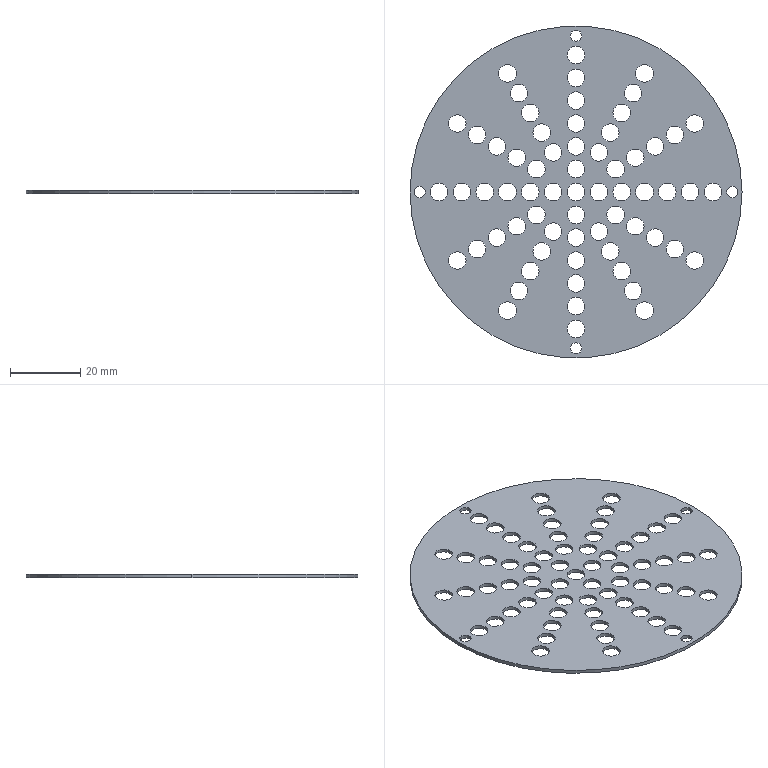Part | SolidWorks | features Cut 2, Extrusion 1 | 1 solid | 142 faces | box 94.5 x 94.5 x 1 mm | volume 5705 mm3 | cylinder 140 | plane 2 | commonest cylinder face diameters 5 x130 3.2 x8 94.5 x2